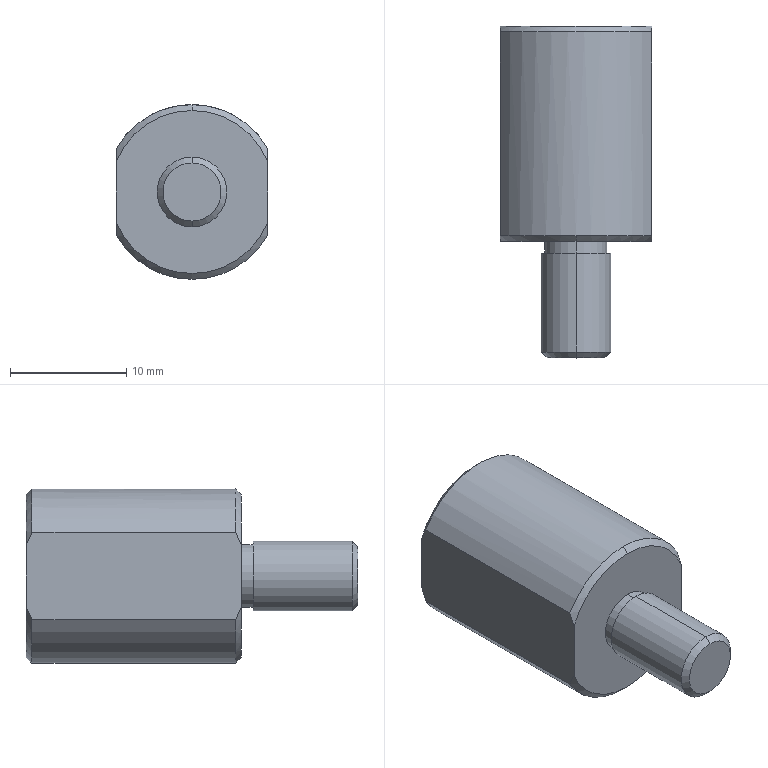Part | STEP file | PN_0003 | 1 solid | 21 faces | box 13 x 28.5 x 15 mm | volume 3349 mm3 | cone 8 | cylinder 7 | plane 6 | commonest cylinder face diameters 15 x3 5.4 x2 6 x2